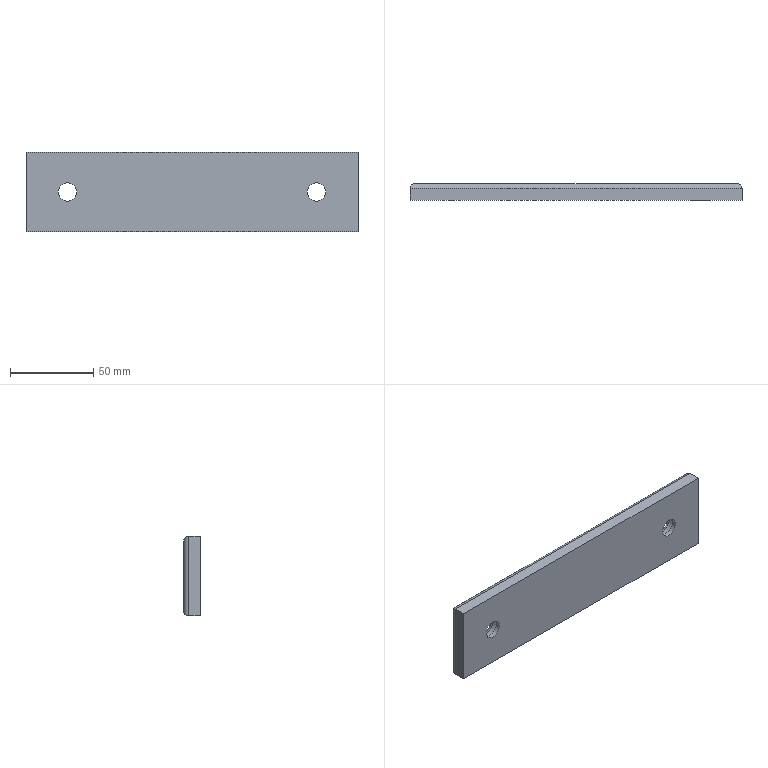Part | STEP file | lll_id4966_x_t | 1 solid | 150 faces | box 200 x 10 x 48 mm | volume 90861 mm3 | plane 102 | other 38 | cylinder 8 | torus 2 | commonest cylinder face diameters 6 x4 11 x2 17.5 x2